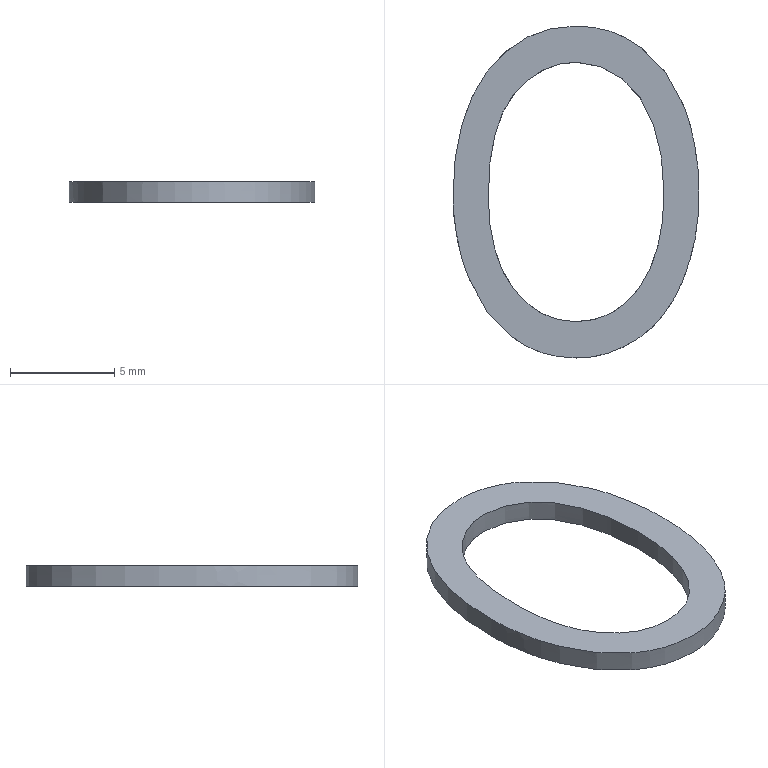Part | STEP file | lll_id982_x_t | 1 solid | 4 faces | box 11.813 x 15.95 x 1 mm | volume 65.616 mm3 | other 2 | plane 2